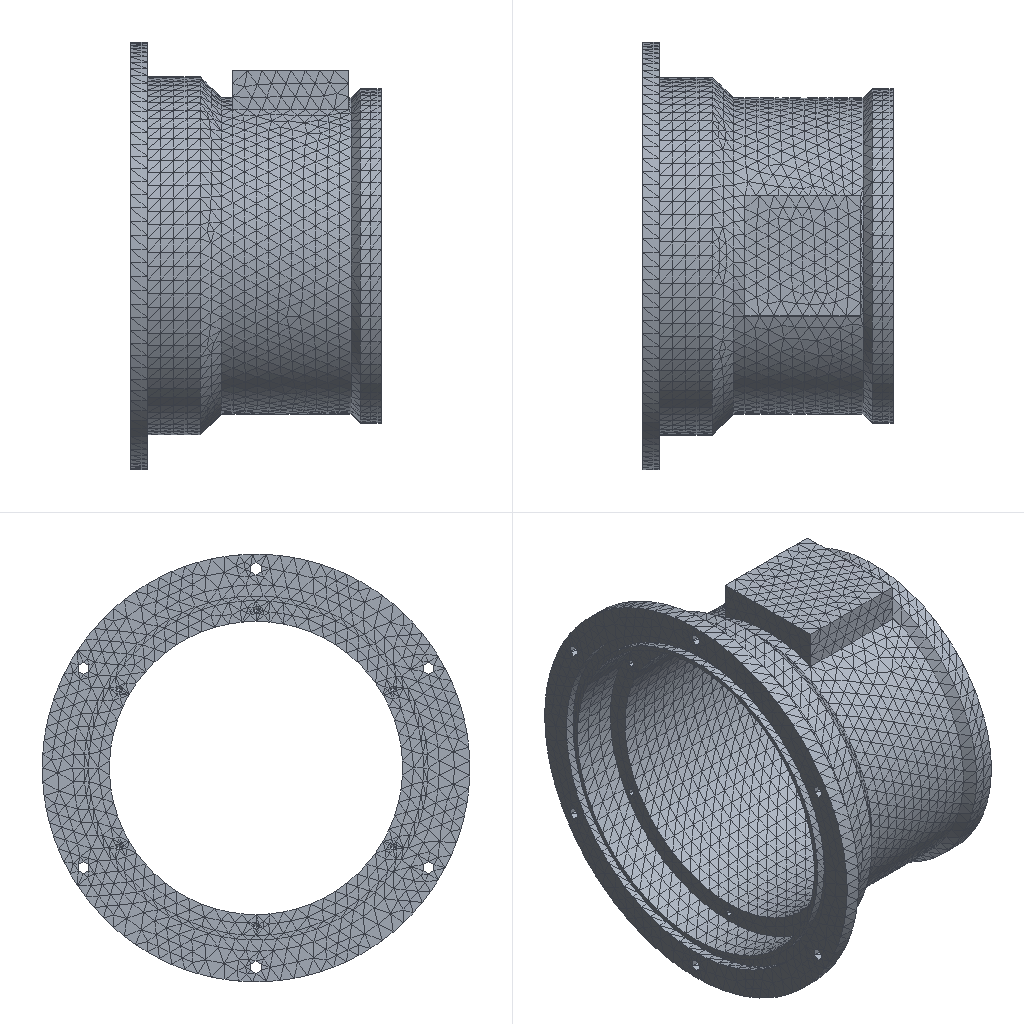Simulation study | nx simcenter
Set-up summary:
category,name,step,type,value,unit,region
solver,nx_nastran (Simcenter)
units,not stated in the deck,,not stated
analysis,deck,,static,static
analysis,solution,,SOL,101
load_step,SUBCASE 1,1,SUBCASE,SPC=1 LOAD=2
load_step,requested,,,1
mesh,nodes,,,28264
mesh,elements,,,14371
element_type,CTETRA,,solid,14371
load,nodal force total,,FX,0.0,model units
load,nodal force total,,FY,0.0,model units
load,nodal force total,,FZ,-2999999.99,model units
load,load commands in deck,,count,272
bc,support commands in deck,,count,1282
analysis,NX solution 0,,Structural,Linear Statics - Single Constraint
check,setup vs results,,match,every grid point's frame and coordinates and every element id; grid points of CTETRA elements
Nastran input file, long lists of numbers shortened:
$*$$$$$$$$$$$$$$$$$$$$$$$$$$$$$$$$$$$$$$$$$$$$$$$$$$$$$$$$$$$$$$$$$
$*
$*                    NX v10.0.0.24 TRANSLATOR
$*                    FOR NX NASTRAN VERSION 10.0
$ (33 more lines like these left out)
ASSIGN OUTPUT2='149_sim1-solution_1.op2' UNIT=12
$*
$*$$$$$$$$$$$$$$$$$$$$$$$$$$$$$$$$$$$
$*
$* EXECUTIVE CONTROL
$*
$*$$$$$$$$$$$$$$$$$$$$$$$$$$$$$$$$$$$
$*
ID,NASTRAN,149_sim1-solution_1
SOL 101
CEND
$*
$*$$$$$$$$$$$$$$$$$$$$$$$$$$$$$$$$$$$
$*
$* CASE CONTROL
$*
$*$$$$$$$$$$$$$$$$$$$$$$$$$$$$$$$$$$$
$*
TITLE = Solution 1
ECHO = NONE
SPC = 1
OUTPUT
BCRESULTS(TRACTION,FORCE,PLOT) = ALL
DISPLACEMENT(PLOT) = ALL
ESE(PLOT) = ALL
FORCE(PLOT,CORNER) = ALL
OLOAD(PLOT) = ALL
SPCFORCES(PLOT) = ALL
STRAIN(PLOT,FIBER,CORNER) = ALL
STRESS(PLOT,CORNER) = ALL
$*  NX Step: Subcase - Static Loads 1
SUBCASE 1
LABEL = Subcase - Static Loads 1
LOAD = 2
$*
$*$$$$$$$$$$$$$$$$$$$$$$$$$$$$$$$$$$$
$*
$* BULK DATA
$*
$*$$$$$$$$$$$$$$$$$$$$$$$$$$$$$$$$$$$
$*
BEGIN BULK
$*
$* PARAM CARDS
$*
PARAM      K6ROT100.0000
PARAM     OIBULK     YES
PARAM    OMACHPR     YES
PARAM       POST      -2
PARAM    POSTEXT     YES
PARAM    UNITSYS   MN-MM
$*
$* GRID CARDS
$*
GRID*              28213               0-1.800000000E+019.2250000000E+01+
*       5.6486831543E-15               0
GRID*              28214               0-1.800000000E+017.9049995422E+01+
*       4.8404163639E-15               0
$ (56524 more lines like these left out)
$*
$* ELEMENT CARDS
$*
$*  NX Mesh Collector: Solid(1)
$*  NX Mesh: 3d_mesh(1)
CTETRA         1       1       1   17654   17655   17589     241   19966+
+            242     243   19965   19967
CTETRA         2       1   23441       2   23331   28195     244     245+
+            246   23463     247     248
$ (28738 more lines like these left out)
$*
$* PROPERTY CARDS
$*
$*  NX Property: PSOLID1
PSOLID         1       1       0                           SMECH
$*
$* MATERIAL CARDS
$*
$*  NX Material: ZL114A
MAT1           17.1000+7        0.3300002.6850-62.5000-5
$*
$* LOAD AND CONSTRAINT CARDS
$*
$*  NX Load and Constraint: Fixed(1)
SPC            1   10369  123456  0.0000
SPC            1   10370  123456  0.0000
SPC            1   10371  123456  0.0000
SPC            1   10372  123456  0.0000
$ (1278 more lines like these left out)
$*  NX Load and Constraint: Force(1)
FORCE          2   12760       011243.90  0.0000  0.0000-1.00000
FORCE          2   12761       011317.41  0.0000  0.0000-1.00000
FORCE          2   12762       011249.49  0.0000  0.0000-1.00000
FORCE          2   12763       011220.62  0.0000  0.0000-1.00000
$ (268 more lines like these left out)
ENDDATA 7653f9c1
Results summary:
result,analysis,,,static
result,last_loadstep,,,1
result,primary field,,,displacements
result,reaction total,,FX,-0.02045,model units
result,reaction total,,FY,-0.3234,model units
result,reaction total,,FZ,3000000.5,model units
result,NX solution 0,,loadcases,1,mm